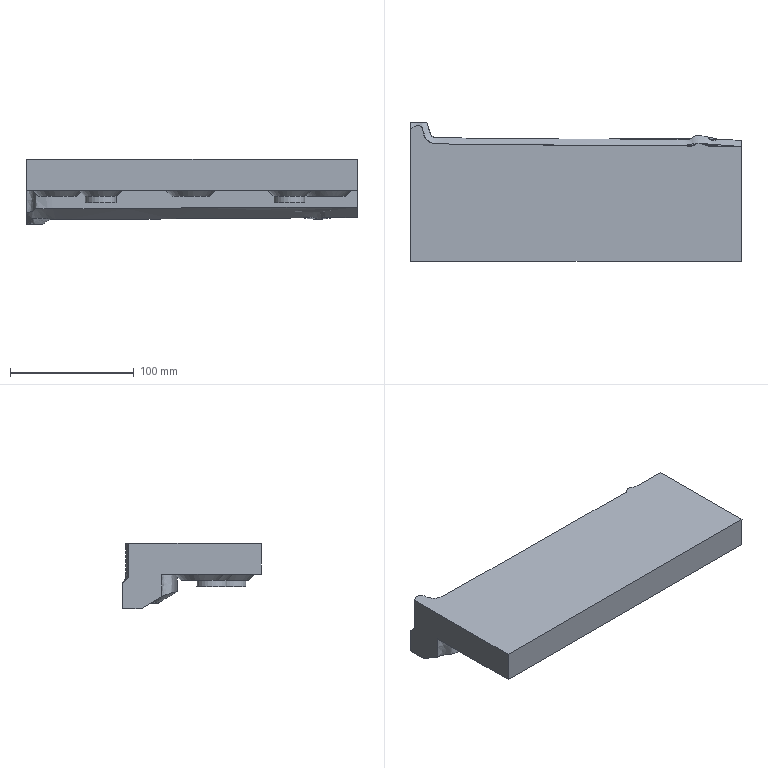Part | NX | features solid 2 | 1 solid | 25 faces | box 267.776 x 112.333 x 52.792 mm | volume 855200 mm3 | plane 11 | spline 7 | cone 5 | cylinder 2 | commonest cylinder face diameters 25 x2